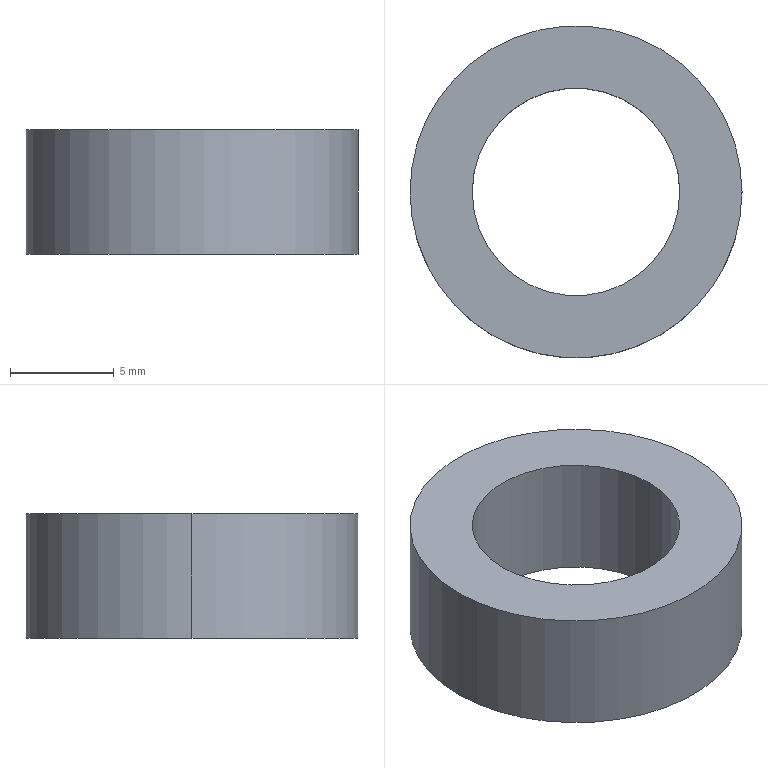Part | STEP file | X77-02004 | 1 solid | 6 faces | box 16 x 16 x 6 mm | volume 735.133 mm3 | cylinder 4 | plane 2 | commonest cylinder face diameters 10 x2 16 x2
STEP:
#1=CARTESIAN_POINT('',(-5.,0.,6.));
#2=VERTEX_POINT('',#1);
#3=CARTESIAN_POINT('',(5.,0.,6.));
#4=VERTEX_POINT('',#3);
#5=CARTESIAN_POINT('',(0.,0.,6.));
#6=DIRECTION('',(0.,0.,1.));
#7=DIRECTION('',(1.,0.,0.));
#8=AXIS2_PLACEMENT_3D('',#5,#6,#7);
#9=CIRCLE('',#8,5.);
#10=EDGE_CURVE('',#2,#4,#9,.T.);
#11=ORIENTED_EDGE('',*,*,#10,.T.);
#12=CARTESIAN_POINT('',(5.,0.,0.));
#13=VERTEX_POINT('',#12);
#14=CARTESIAN_POINT('',(5.,0.,6.));
#15=DIRECTION('',(0.,0.,-1.));
#16=VECTOR('',#15,1000.);
#17=LINE('',#14,#16);
#18=EDGE_CURVE('',#4,#13,#17,.T.);
#19=ORIENTED_EDGE('',*,*,#18,.T.);
#20=CARTESIAN_POINT('',(-5.,0.,0.));
#21=VERTEX_POINT('',#20);
#22=CARTESIAN_POINT('',(0.,0.,0.));
#23=DIRECTION('',(0.,0.,1.));
#24=DIRECTION('',(1.,0.,0.));
#25=AXIS2_PLACEMENT_3D('',#22,#23,#24);
#26=CIRCLE('',#25,5.);
#27=EDGE_CURVE('',#21,#13,#26,.T.);
#28=ORIENTED_EDGE('',*,*,#27,.F.);
#29=CARTESIAN_POINT('',(-5.,0.,6.));
#30=DIRECTION('',(0.,0.,-1.));
#31=VECTOR('',#30,1000.);
#32=LINE('',#29,#31);
#33=EDGE_CURVE('',#2,#21,#32,.T.);
#34=ORIENTED_EDGE('',*,*,#33,.F.);
#35=EDGE_LOOP('',(#11,#19,#28,#34));
#36=FACE_OUTER_BOUND('',#35,.T.);
#37=CARTESIAN_POINT('',(0.,0.,6.));
#38=DIRECTION('',(0.,0.,-1.));
#39=DIRECTION('',(-1.,0.,0.));
#40=AXIS2_PLACEMENT_3D('',#37,#38,#39);
#41=CYLINDRICAL_SURFACE('',#40,5.);
#42=ADVANCED_FACE('',(#36),#41,.F.);
#43=CARTESIAN_POINT('',(8.,0.,6.));
#44=VERTEX_POINT('',#43);
#45=CARTESIAN_POINT('',(-8.,0.,6.));
#46=VERTEX_POINT('',#45);
#47=CARTESIAN_POINT('',(0.,0.,6.));
#48=DIRECTION('',(0.,0.,1.));
#49=DIRECTION('',(1.,0.,0.));
#50=AXIS2_PLACEMENT_3D('',#47,#48,#49);
#51=CIRCLE('',#50,8.);
#52=EDGE_CURVE('',#44,#46,#51,.T.);
#53=ORIENTED_EDGE('',*,*,#52,.F.);
#54=CARTESIAN_POINT('',(8.,0.,0.));
#55=VERTEX_POINT('',#54);
#56=CARTESIAN_POINT('',(8.,0.,6.));
#57=DIRECTION('',(0.,0.,-1.));
#58=VECTOR('',#57,1000.);
#59=LINE('',#56,#58);
#60=EDGE_CURVE('',#44,#55,#59,.T.);
#61=ORIENTED_EDGE('',*,*,#60,.T.);
#62=CARTESIAN_POINT('',(-8.,0.,0.));
#63=VERTEX_POINT('',#62);
#64=CARTESIAN_POINT('',(0.,0.,0.));
#65=DIRECTION('',(0.,0.,1.));
#66=DIRECTION('',(1.,0.,0.));
#67=AXIS2_PLACEMENT_3D('',#64,#65,#66);
#68=CIRCLE('',#67,8.);
#69=EDGE_CURVE('',#55,#63,#68,.T.);
#70=ORIENTED_EDGE('',*,*,#69,.T.);
#71=CARTESIAN_POINT('',(-8.,0.,6.));
#72=DIRECTION('',(0.,0.,-1.));
#73=VECTOR('',#72,1000.);
#74=LINE('',#71,#73);
#75=EDGE_CURVE('',#46,#63,#74,.T.);
#76=ORIENTED_EDGE('',*,*,#75,.F.);
#77=EDGE_LOOP('',(#53,#61,#70,#76));
#78=FACE_OUTER_BOUND('',#77,.T.);
#79=CARTESIAN_POINT('',(0.,0.,6.));
#80=DIRECTION('',(0.,0.,-1.));
#81=DIRECTION('',(-1.,0.,0.));
#82=AXIS2_PLACEMENT_3D('',#79,#80,#81);
#83=CYLINDRICAL_SURFACE('',#82,8.);
#84=ADVANCED_FACE('',(#78),#83,.T.);
#85=CARTESIAN_POINT('',(0.,0.,6.));
#86=DIRECTION('',(0.,0.,1.));
#87=DIRECTION('',(1.,0.,0.));
#88=AXIS2_PLACEMENT_3D('',#85,#86,#87);
#89=CIRCLE('',#88,8.);
#90=EDGE_CURVE('',#46,#44,#89,.T.);
#91=ORIENTED_EDGE('',*,*,#90,.T.);
#92=ORIENTED_EDGE('',*,*,#52,.T.);
#93=EDGE_LOOP('',(#91,#92));
#94=FACE_OUTER_BOUND('',#93,.T.);
#95=ORIENTED_EDGE('',*,*,#10,.F.);
#96=CARTESIAN_POINT('',(0.,0.,6.));
#97=DIRECTION('',(0.,0.,1.));
#98=DIRECTION('',(1.,0.,0.));
#99=AXIS2_PLACEMENT_3D('',#96,#97,#98);
#100=CIRCLE('',#99,5.);
#101=EDGE_CURVE('',#4,#2,#100,.T.);
#102=ORIENTED_EDGE('',*,*,#101,.F.);
#103=EDGE_LOOP('',(#95,#102));
#104=FACE_BOUND('',#103,.T.);
#105=CARTESIAN_POINT('',(0.,0.,6.));
#106=DIRECTION('',(0.,0.,1.));
#107=DIRECTION('',(1.,0.,0.));
#108=AXIS2_PLACEMENT_3D('',#105,#106,#107);
#109=PLANE('',#108);
#110=ADVANCED_FACE('',(#94,#104),#109,.T.);
#111=CARTESIAN_POINT('',(0.,0.,0.));
#112=DIRECTION('',(0.,0.,1.));
#113=DIRECTION('',(1.,0.,0.));
#114=AXIS2_PLACEMENT_3D('',#111,#112,#113);
#115=CIRCLE('',#114,8.);
#116=EDGE_CURVE('',#63,#55,#115,.T.);
#117=ORIENTED_EDGE('',*,*,#116,.F.);
#118=ORIENTED_EDGE('',*,*,#69,.F.);
#119=EDGE_LOOP('',(#117,#118));
#120=FACE_OUTER_BOUND('',#119,.T.);
#121=ORIENTED_EDGE('',*,*,#27,.T.);
#122=CARTESIAN_POINT('',(0.,0.,0.));
#123=DIRECTION('',(0.,0.,1.));
#124=DIRECTION('',(1.,0.,0.));
#125=AXIS2_PLACEMENT_3D('',#122,#123,#124);
#126=CIRCLE('',#125,5.);
#127=EDGE_CURVE('',#13,#21,#126,.T.);
#128=ORIENTED_EDGE('',*,*,#127,.T.);
#129=EDGE_LOOP('',(#121,#128));
#130=FACE_BOUND('',#129,.T.);
#131=CARTESIAN_POINT('',(0.,0.,0.));
#132=DIRECTION('',(0.,0.,1.));
#133=DIRECTION('',(1.,0.,0.));
#134=AXIS2_PLACEMENT_3D('',#131,#132,#133);
#135=PLANE('',#134);
#136=ADVANCED_FACE('',(#120,#130),#135,.F.);
#137=ORIENTED_EDGE('',*,*,#60,.F.);
#138=ORIENTED_EDGE('',*,*,#90,.F.);
#139=ORIENTED_EDGE('',*,*,#75,.T.);
#140=ORIENTED_EDGE('',*,*,#116,.T.);
#141=EDGE_LOOP('',(#137,#138,#139,#140));
#142=FACE_OUTER_BOUND('',#141,.T.);
#143=CARTESIAN_POINT('',(0.,0.,6.));
#144=DIRECTION('',(0.,0.,-1.));
#145=DIRECTION('',(-1.,0.,0.));
#146=AXIS2_PLACEMENT_3D('',#143,#144,#145);
#147=CYLINDRICAL_SURFACE('',#146,8.);
#148=ADVANCED_FACE('',(#142),#147,.T.);
#149=ORIENTED_EDGE('',*,*,#18,.F.);
#150=ORIENTED_EDGE('',*,*,#101,.T.);
#151=ORIENTED_EDGE('',*,*,#33,.T.);
#152=ORIENTED_EDGE('',*,*,#127,.F.);
#153=EDGE_LOOP('',(#149,#150,#151,#152));
#154=FACE_OUTER_BOUND('',#153,.T.);
#155=CARTESIAN_POINT('',(0.,0.,6.));
#156=DIRECTION('',(0.,0.,-1.));
#157=DIRECTION('',(-1.,0.,0.));
#158=AXIS2_PLACEMENT_3D('',#155,#156,#157);
#159=CYLINDRICAL_SURFACE('',#158,5.);
#160=ADVANCED_FACE('',(#154),#159,.F.);
#161=CLOSED_SHELL('',(#42,#84,#110,#136,#148,#160));
#162=MANIFOLD_SOLID_BREP('',#161);
#163=CARTESIAN_POINT('',(0.,0.,0.));
#164=DIRECTION('',(0.,0.,1.));
#165=DIRECTION('',(1.,0.,0.));
#166=AXIS2_PLACEMENT_3D('',#163,#164,#165);
#167=(LENGTH_UNIT()NAMED_UNIT(*)SI_UNIT(.MILLI.,.METRE.));
#168=UNCERTAINTY_MEASURE_WITH_UNIT(LENGTH_MEASURE(0.00001),#167,'','');
#169=(NAMED_UNIT(*)PLANE_ANGLE_UNIT()SI_UNIT($,.RADIAN.));
#170=(NAMED_UNIT(*)SI_UNIT($,.STERADIAN.)SOLID_ANGLE_UNIT());
#171=(GEOMETRIC_REPRESENTATION_CONTEXT(3)GLOBAL_UNCERTAINTY_ASSIGNED_CONTEXT((#168))GLOBAL_UNIT_ASSIGNED_CONTEXT((#167,#169,#170))REPRESENTATION_CONTEXT('',''));
#172=ADVANCED_BREP_SHAPE_REPRESENTATION('',(#162,#166),#171);